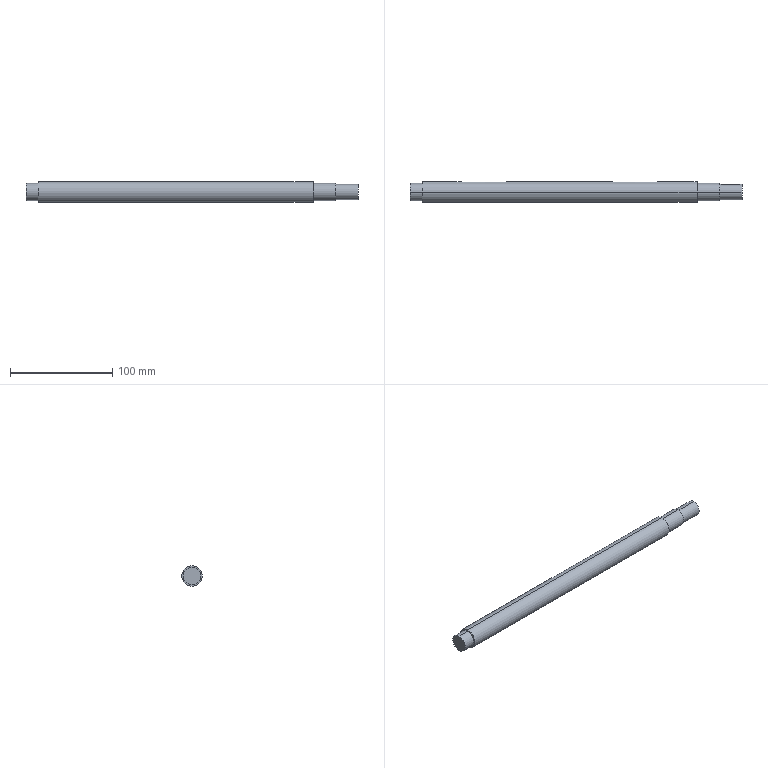Part | STEP file | PN_0012 (main rotating shaft) | 1 solid | 28 faces | box 325 x 20 x 20 mm | volume 94666 mm3 | cylinder 14 | plane 14 | commonest cylinder face diameters 5 x4 17 x4 4 x2 15 x2 20 x2